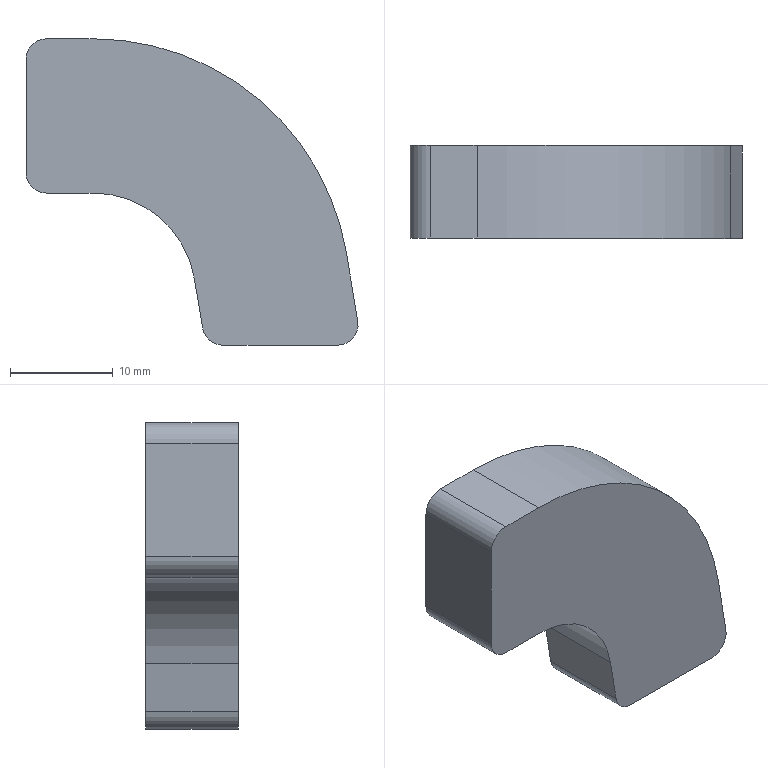Part | SolidWorks | features Fillet 1, FlatPattern 1, SMBaseFlange 1, SheetMetal 1 | 1 solid | 14 faces | box 32.296 x 9 x 29.799 mm | volume 5219 mm3 | plane 8 | cylinder 6 | commonest cylinder face diameters 4 x4 20 x1 50 x1
STEP:
#1=CARTESIAN_POINT('',(0.,0.,2.));
#2=VERTEX_POINT('',#1);
#3=CARTESIAN_POINT('',(0.,0.,13.));
#4=VERTEX_POINT('',#3);
#5=CARTESIAN_POINT('',(0.,0.,0.));
#6=DIRECTION('',(0.,0.,1.));
#7=VECTOR('',#6,1000.);
#8=LINE('',#5,#7);
#9=EDGE_CURVE('',#2,#4,#8,.T.);
#10=ORIENTED_EDGE('',*,*,#9,.T.);
#11=CARTESIAN_POINT('',(0.,9.,13.));
#12=VERTEX_POINT('',#11);
#13=CARTESIAN_POINT('',(0.,9.,13.));
#14=DIRECTION('',(0.,1.,0.));
#15=VECTOR('',#14,1000.);
#16=LINE('',#13,#15);
#17=EDGE_CURVE('',#4,#12,#16,.T.);
#18=ORIENTED_EDGE('',*,*,#17,.T.);
#19=CARTESIAN_POINT('',(0.,9.,2.));
#20=VERTEX_POINT('',#19);
#21=CARTESIAN_POINT('',(0.,9.,0.));
#22=DIRECTION('',(0.,0.,1.));
#23=VECTOR('',#22,1000.);
#24=LINE('',#21,#23);
#25=EDGE_CURVE('',#20,#12,#24,.T.);
#26=ORIENTED_EDGE('',*,*,#25,.F.);
#27=CARTESIAN_POINT('',(0.,9.,2.));
#28=DIRECTION('',(0.,-1.,0.));
#29=VECTOR('',#28,1000.);
#30=LINE('',#27,#29);
#31=EDGE_CURVE('',#20,#2,#30,.T.);
#32=ORIENTED_EDGE('',*,*,#31,.T.);
#33=EDGE_LOOP('',(#10,#18,#26,#32));
#34=FACE_OUTER_BOUND('',#33,.T.);
#35=CARTESIAN_POINT('',(0.,9.,0.));
#36=DIRECTION('',(1.,0.,0.));
#37=DIRECTION('',(0.,0.,-1.));
#38=AXIS2_PLACEMENT_3D('',#35,#36,#37);
#39=PLANE('',#38);
#40=ADVANCED_FACE('',(#34),#39,.F.);
#41=CARTESIAN_POINT('',(2.,9.,15.));
#42=VERTEX_POINT('',#41);
#43=CARTESIAN_POINT('',(6.519,9.,15.));
#44=VERTEX_POINT('',#43);
#45=CARTESIAN_POINT('',(0.,9.,15.));
#46=DIRECTION('',(1.,0.,0.));
#47=VECTOR('',#46,1000.);
#48=LINE('',#45,#47);
#49=EDGE_CURVE('',#42,#44,#48,.T.);
#50=ORIENTED_EDGE('',*,*,#49,.F.);
#51=CARTESIAN_POINT('',(2.,0.,15.));
#52=VERTEX_POINT('',#51);
#53=CARTESIAN_POINT('',(2.,9.,15.));
#54=DIRECTION('',(0.,-1.,0.));
#55=VECTOR('',#54,1000.);
#56=LINE('',#53,#55);
#57=EDGE_CURVE('',#42,#52,#56,.T.);
#58=ORIENTED_EDGE('',*,*,#57,.T.);
#59=CARTESIAN_POINT('',(6.519,0.,15.));
#60=VERTEX_POINT('',#59);
#61=CARTESIAN_POINT('',(0.,0.,15.));
#62=DIRECTION('',(1.,0.,0.));
#63=VECTOR('',#62,1000.);
#64=LINE('',#61,#63);
#65=EDGE_CURVE('',#52,#60,#64,.T.);
#66=ORIENTED_EDGE('',*,*,#65,.T.);
#67=CARTESIAN_POINT('',(6.519,9.,15.));
#68=DIRECTION('',(0.,-1.,0.));
#69=VECTOR('',#68,1000.);
#70=LINE('',#67,#69);
#71=EDGE_CURVE('',#44,#60,#70,.T.);
#72=ORIENTED_EDGE('',*,*,#71,.F.);
#73=EDGE_LOOP('',(#50,#58,#66,#72));
#74=FACE_OUTER_BOUND('',#73,.T.);
#75=CARTESIAN_POINT('',(0.,9.,15.));
#76=DIRECTION('',(0.,0.,-1.));
#77=DIRECTION('',(-1.,0.,0.));
#78=AXIS2_PLACEMENT_3D('',#75,#76,#77);
#79=PLANE('',#78);
#80=ADVANCED_FACE('',(#74),#79,.F.);
#81=CARTESIAN_POINT('',(31.184,0.,-5.917));
#82=VERTEX_POINT('',#81);
#83=CARTESIAN_POINT('',(6.519,0.,-10.));
#84=DIRECTION('',(0.,1.,0.));
#85=DIRECTION('',(0.,0.,1.));
#86=AXIS2_PLACEMENT_3D('',#83,#84,#85);
#87=CIRCLE('',#86,25.);
#88=EDGE_CURVE('',#60,#82,#87,.T.);
#89=ORIENTED_EDGE('',*,*,#88,.T.);
#90=CARTESIAN_POINT('',(31.184,9.,-5.917));
#91=VERTEX_POINT('',#90);
#92=CARTESIAN_POINT('',(31.184,9.,-5.917));
#93=DIRECTION('',(0.,-1.,0.));
#94=VECTOR('',#93,1000.);
#95=LINE('',#92,#94);
#96=EDGE_CURVE('',#91,#82,#95,.T.);
#97=ORIENTED_EDGE('',*,*,#96,.F.);
#98=CARTESIAN_POINT('',(6.519,9.,-10.));
#99=DIRECTION('',(0.,1.,0.));
#100=DIRECTION('',(0.,0.,1.));
#101=AXIS2_PLACEMENT_3D('',#98,#99,#100);
#102=CIRCLE('',#101,25.);
#103=EDGE_CURVE('',#44,#91,#102,.T.);
#104=ORIENTED_EDGE('',*,*,#103,.F.);
#105=ORIENTED_EDGE('',*,*,#71,.T.);
#106=EDGE_LOOP('',(#89,#97,#104,#105));
#107=FACE_OUTER_BOUND('',#106,.T.);
#108=CARTESIAN_POINT('',(6.519,9.,-10.));
#109=DIRECTION('',(0.,-1.,0.));
#110=DIRECTION('',(0.,0.,-1.));
#111=AXIS2_PLACEMENT_3D('',#108,#109,#110);
#112=CYLINDRICAL_SURFACE('',#111,25.);
#113=ADVANCED_FACE('',(#107),#112,.T.);
#114=CARTESIAN_POINT('',(32.269,0.,-12.472));
#115=VERTEX_POINT('',#114);
#116=CARTESIAN_POINT('',(31.184,0.,-5.917));
#117=DIRECTION('',(0.1633,0.,-0.9866));
#118=VECTOR('',#117,1000.);
#119=LINE('',#116,#118);
#120=EDGE_CURVE('',#82,#115,#119,.T.);
#121=ORIENTED_EDGE('',*,*,#120,.T.);
#122=CARTESIAN_POINT('',(32.269,9.,-12.472));
#123=VERTEX_POINT('',#122);
#124=CARTESIAN_POINT('',(32.269,9.,-12.472));
#125=DIRECTION('',(0.,1.,0.));
#126=VECTOR('',#125,1000.);
#127=LINE('',#124,#126);
#128=EDGE_CURVE('',#115,#123,#127,.T.);
#129=ORIENTED_EDGE('',*,*,#128,.T.);
#130=CARTESIAN_POINT('',(31.184,9.,-5.917));
#131=DIRECTION('',(0.1633,0.,-0.9866));
#132=VECTOR('',#131,1000.);
#133=LINE('',#130,#132);
#134=EDGE_CURVE('',#91,#123,#133,.T.);
#135=ORIENTED_EDGE('',*,*,#134,.F.);
#136=ORIENTED_EDGE('',*,*,#96,.T.);
#137=EDGE_LOOP('',(#121,#129,#135,#136));
#138=FACE_OUTER_BOUND('',#137,.T.);
#139=CARTESIAN_POINT('',(31.184,9.,-5.917));
#140=DIRECTION('',(-0.9866,0.,-0.1633));
#141=DIRECTION('',(-0.1633,0.,0.9866));
#142=AXIS2_PLACEMENT_3D('',#139,#140,#141);
#143=PLANE('',#142);
#144=ADVANCED_FACE('',(#138),#143,.F.);
#145=CARTESIAN_POINT('',(30.296,9.,-14.799));
#146=VERTEX_POINT('',#145);
#147=CARTESIAN_POINT('',(19.146,9.,-14.799));
#148=VERTEX_POINT('',#147);
#149=CARTESIAN_POINT('',(17.45,9.,-14.799));
#150=DIRECTION('',(-1.,0.,0.));
#151=VECTOR('',#150,1000.);
#152=LINE('',#149,#151);
#153=EDGE_CURVE('',#146,#148,#152,.T.);
#154=ORIENTED_EDGE('',*,*,#153,.F.);
#155=CARTESIAN_POINT('',(30.296,0.,-14.799));
#156=VERTEX_POINT('',#155);
#157=CARTESIAN_POINT('',(30.296,9.,-14.799));
#158=DIRECTION('',(0.,-1.,0.));
#159=VECTOR('',#158,1000.);
#160=LINE('',#157,#159);
#161=EDGE_CURVE('',#146,#156,#160,.T.);
#162=ORIENTED_EDGE('',*,*,#161,.T.);
#163=CARTESIAN_POINT('',(19.146,0.,-14.799));
#164=VERTEX_POINT('',#163);
#165=CARTESIAN_POINT('',(17.45,0.,-14.799));
#166=DIRECTION('',(-1.,0.,0.));
#167=VECTOR('',#166,1000.);
#168=LINE('',#165,#167);
#169=EDGE_CURVE('',#156,#164,#168,.T.);
#170=ORIENTED_EDGE('',*,*,#169,.T.);
#171=CARTESIAN_POINT('',(19.146,9.,-14.799));
#172=DIRECTION('',(0.,1.,0.));
#173=VECTOR('',#172,1000.);
#174=LINE('',#171,#173);
#175=EDGE_CURVE('',#164,#148,#174,.T.);
#176=ORIENTED_EDGE('',*,*,#175,.T.);
#177=EDGE_LOOP('',(#154,#162,#170,#176));
#178=FACE_OUTER_BOUND('',#177,.T.);
#179=CARTESIAN_POINT('',(17.45,9.,-14.799));
#180=DIRECTION('',(0.,0.,1.));
#181=DIRECTION('',(1.,0.,0.));
#182=AXIS2_PLACEMENT_3D('',#179,#180,#181);
#183=PLANE('',#182);
#184=ADVANCED_FACE('',(#178),#183,.F.);
#185=CARTESIAN_POINT('',(17.173,9.,-13.125));
#186=VERTEX_POINT('',#185);
#187=CARTESIAN_POINT('',(16.385,9.,-8.367));
#188=VERTEX_POINT('',#187);
#189=CARTESIAN_POINT('',(16.385,9.,-8.367));
#190=DIRECTION('',(-0.1633,0.,0.9866));
#191=VECTOR('',#190,1000.);
#192=LINE('',#189,#191);
#193=EDGE_CURVE('',#186,#188,#192,.T.);
#194=ORIENTED_EDGE('',*,*,#193,.F.);
#195=CARTESIAN_POINT('',(17.173,0.,-13.125));
#196=VERTEX_POINT('',#195);
#197=CARTESIAN_POINT('',(17.173,9.,-13.125));
#198=DIRECTION('',(0.,-1.,0.));
#199=VECTOR('',#198,1000.);
#200=LINE('',#197,#199);
#201=EDGE_CURVE('',#186,#196,#200,.T.);
#202=ORIENTED_EDGE('',*,*,#201,.T.);
#203=CARTESIAN_POINT('',(16.385,0.,-8.367));
#204=VERTEX_POINT('',#203);
#205=CARTESIAN_POINT('',(16.385,0.,-8.367));
#206=DIRECTION('',(-0.1633,0.,0.9866));
#207=VECTOR('',#206,1000.);
#208=LINE('',#205,#207);
#209=EDGE_CURVE('',#196,#204,#208,.T.);
#210=ORIENTED_EDGE('',*,*,#209,.T.);
#211=CARTESIAN_POINT('',(16.385,9.,-8.367));
#212=DIRECTION('',(0.,-1.,0.));
#213=VECTOR('',#212,1000.);
#214=LINE('',#211,#213);
#215=EDGE_CURVE('',#188,#204,#214,.T.);
#216=ORIENTED_EDGE('',*,*,#215,.F.);
#217=EDGE_LOOP('',(#194,#202,#210,#216));
#218=FACE_OUTER_BOUND('',#217,.T.);
#219=CARTESIAN_POINT('',(16.385,9.,-8.367));
#220=DIRECTION('',(0.9866,0.,0.1633));
#221=DIRECTION('',(0.1633,0.,-0.9866));
#222=AXIS2_PLACEMENT_3D('',#219,#220,#221);
#223=PLANE('',#222);
#224=ADVANCED_FACE('',(#218),#223,.F.);
#225=CARTESIAN_POINT('',(6.519,0.,0.));
#226=VERTEX_POINT('',#225);
#227=CARTESIAN_POINT('',(6.519,0.,-10.));
#228=DIRECTION('',(0.,-1.,0.));
#229=DIRECTION('',(0.,0.,1.));
#230=AXIS2_PLACEMENT_3D('',#227,#228,#229);
#231=CIRCLE('',#230,10.);
#232=EDGE_CURVE('',#204,#226,#231,.T.);
#233=ORIENTED_EDGE('',*,*,#232,.T.);
#234=CARTESIAN_POINT('',(6.519,9.,0.));
#235=VERTEX_POINT('',#234);
#236=CARTESIAN_POINT('',(6.519,9.,0.));
#237=DIRECTION('',(0.,-1.,0.));
#238=VECTOR('',#237,1000.);
#239=LINE('',#236,#238);
#240=EDGE_CURVE('',#235,#226,#239,.T.);
#241=ORIENTED_EDGE('',*,*,#240,.F.);
#242=CARTESIAN_POINT('',(6.519,9.,-10.));
#243=DIRECTION('',(0.,-1.,0.));
#244=DIRECTION('',(0.,0.,1.));
#245=AXIS2_PLACEMENT_3D('',#242,#243,#244);
#246=CIRCLE('',#245,10.);
#247=EDGE_CURVE('',#188,#235,#246,.T.);
#248=ORIENTED_EDGE('',*,*,#247,.F.);
#249=ORIENTED_EDGE('',*,*,#215,.T.);
#250=EDGE_LOOP('',(#233,#241,#248,#249));
#251=FACE_OUTER_BOUND('',#250,.T.);
#252=CARTESIAN_POINT('',(6.519,9.,-10.));
#253=DIRECTION('',(0.,-1.,0.));
#254=DIRECTION('',(0.,0.,-1.));
#255=AXIS2_PLACEMENT_3D('',#252,#253,#254);
#256=CYLINDRICAL_SURFACE('',#255,10.);
#257=ADVANCED_FACE('',(#251),#256,.F.);
#258=CARTESIAN_POINT('',(2.,0.,0.));
#259=VERTEX_POINT('',#258);
#260=CARTESIAN_POINT('',(0.,0.,0.));
#261=DIRECTION('',(-1.,0.,0.));
#262=VECTOR('',#261,1000.);
#263=LINE('',#260,#262);
#264=EDGE_CURVE('',#226,#259,#263,.T.);
#265=ORIENTED_EDGE('',*,*,#264,.T.);
#266=CARTESIAN_POINT('',(2.,9.,0.));
#267=VERTEX_POINT('',#266);
#268=CARTESIAN_POINT('',(2.,9.,0.));
#269=DIRECTION('',(0.,1.,0.));
#270=VECTOR('',#269,1000.);
#271=LINE('',#268,#270);
#272=EDGE_CURVE('',#259,#267,#271,.T.);
#273=ORIENTED_EDGE('',*,*,#272,.T.);
#274=CARTESIAN_POINT('',(0.,9.,0.));
#275=DIRECTION('',(-1.,0.,0.));
#276=VECTOR('',#275,1000.);
#277=LINE('',#274,#276);
#278=EDGE_CURVE('',#235,#267,#277,.T.);
#279=ORIENTED_EDGE('',*,*,#278,.F.);
#280=ORIENTED_EDGE('',*,*,#240,.T.);
#281=EDGE_LOOP('',(#265,#273,#279,#280));
#282=FACE_OUTER_BOUND('',#281,.T.);
#283=CARTESIAN_POINT('',(0.,9.,0.));
#284=DIRECTION('',(0.,0.,1.));
#285=DIRECTION('',(1.,0.,0.));
#286=AXIS2_PLACEMENT_3D('',#283,#284,#285);
#287=PLANE('',#286);
#288=ADVANCED_FACE('',(#282),#287,.F.);
#289=ORIENTED_EDGE('',*,*,#134,.T.);
#290=CARTESIAN_POINT('',(30.296,9.,-12.799));
#291=DIRECTION('',(0.,1.,0.));
#292=DIRECTION('',(0.,0.,1.));
#293=AXIS2_PLACEMENT_3D('',#290,#291,#292);
#294=CIRCLE('',#293,2.);
#295=EDGE_CURVE('',#123,#146,#294,.T.);
#296=ORIENTED_EDGE('',*,*,#295,.T.);
#297=ORIENTED_EDGE('',*,*,#153,.T.);
#298=CARTESIAN_POINT('',(19.146,9.,-12.799));
#299=DIRECTION('',(0.,1.,0.));
#300=DIRECTION('',(0.,0.,1.));
#301=AXIS2_PLACEMENT_3D('',#298,#299,#300);
#302=CIRCLE('',#301,2.);
#303=EDGE_CURVE('',#148,#186,#302,.T.);
#304=ORIENTED_EDGE('',*,*,#303,.T.);
#305=ORIENTED_EDGE('',*,*,#193,.T.);
#306=ORIENTED_EDGE('',*,*,#247,.T.);
#307=ORIENTED_EDGE('',*,*,#278,.T.);
#308=CARTESIAN_POINT('',(2.,9.,2.));
#309=DIRECTION('',(0.,1.,0.));
#310=DIRECTION('',(0.,0.,1.));
#311=AXIS2_PLACEMENT_3D('',#308,#309,#310);
#312=CIRCLE('',#311,2.);
#313=EDGE_CURVE('',#267,#20,#312,.T.);
#314=ORIENTED_EDGE('',*,*,#313,.T.);
#315=ORIENTED_EDGE('',*,*,#25,.T.);
#316=CARTESIAN_POINT('',(2.,9.,13.));
#317=DIRECTION('',(0.,1.,0.));
#318=DIRECTION('',(0.,0.,1.));
#319=AXIS2_PLACEMENT_3D('',#316,#317,#318);
#320=CIRCLE('',#319,2.);
#321=EDGE_CURVE('',#12,#42,#320,.T.);
#322=ORIENTED_EDGE('',*,*,#321,.T.);
#323=ORIENTED_EDGE('',*,*,#49,.T.);
#324=ORIENTED_EDGE('',*,*,#103,.T.);
#325=EDGE_LOOP('',(#289,#296,#297,#304,#305,#306,#307,#314,#315,#322,#323,#324));
#326=FACE_OUTER_BOUND('',#325,.T.);
#327=CARTESIAN_POINT('',(6.519,9.,-10.));
#328=DIRECTION('',(0.,1.,0.));
#329=DIRECTION('',(0.,0.,1.));
#330=AXIS2_PLACEMENT_3D('',#327,#328,#329);
#331=PLANE('',#330);
#332=ADVANCED_FACE('',(#326),#331,.T.);
#333=ORIENTED_EDGE('',*,*,#169,.F.);
#334=CARTESIAN_POINT('',(30.296,0.,-12.799));
#335=DIRECTION('',(0.,-1.,0.));
#336=DIRECTION('',(0.,0.,1.));
#337=AXIS2_PLACEMENT_3D('',#334,#335,#336);
#338=CIRCLE('',#337,2.);
#339=EDGE_CURVE('',#156,#115,#338,.T.);
#340=ORIENTED_EDGE('',*,*,#339,.T.);
#341=ORIENTED_EDGE('',*,*,#120,.F.);
#342=ORIENTED_EDGE('',*,*,#88,.F.);
#343=ORIENTED_EDGE('',*,*,#65,.F.);
#344=CARTESIAN_POINT('',(2.,0.,13.));
#345=DIRECTION('',(0.,-1.,0.));
#346=DIRECTION('',(0.,0.,1.));
#347=AXIS2_PLACEMENT_3D('',#344,#345,#346);
#348=CIRCLE('',#347,2.);
#349=EDGE_CURVE('',#52,#4,#348,.T.);
#350=ORIENTED_EDGE('',*,*,#349,.T.);
#351=ORIENTED_EDGE('',*,*,#9,.F.);
#352=CARTESIAN_POINT('',(2.,0.,2.));
#353=DIRECTION('',(0.,-1.,0.));
#354=DIRECTION('',(0.,0.,1.));
#355=AXIS2_PLACEMENT_3D('',#352,#353,#354);
#356=CIRCLE('',#355,2.);
#357=EDGE_CURVE('',#2,#259,#356,.T.);
#358=ORIENTED_EDGE('',*,*,#357,.T.);
#359=ORIENTED_EDGE('',*,*,#264,.F.);
#360=ORIENTED_EDGE('',*,*,#232,.F.);
#361=ORIENTED_EDGE('',*,*,#209,.F.);
#362=CARTESIAN_POINT('',(19.146,0.,-12.799));
#363=DIRECTION('',(0.,-1.,0.));
#364=DIRECTION('',(0.,0.,1.));
#365=AXIS2_PLACEMENT_3D('',#362,#363,#364);
#366=CIRCLE('',#365,2.);
#367=EDGE_CURVE('',#196,#164,#366,.T.);
#368=ORIENTED_EDGE('',*,*,#367,.T.);
#369=EDGE_LOOP('',(#333,#340,#341,#342,#343,#350,#351,#358,#359,#360,#361,#368));
#370=FACE_OUTER_BOUND('',#369,.T.);
#371=CARTESIAN_POINT('',(6.519,0.,-10.));
#372=DIRECTION('',(0.,1.,0.));
#373=DIRECTION('',(0.,0.,1.));
#374=AXIS2_PLACEMENT_3D('',#371,#372,#373);
#375=PLANE('',#374);
#376=ADVANCED_FACE('',(#370),#375,.F.);
#377=ORIENTED_EDGE('',*,*,#295,.F.);
#378=ORIENTED_EDGE('',*,*,#128,.F.);
#379=ORIENTED_EDGE('',*,*,#339,.F.);
#380=ORIENTED_EDGE('',*,*,#161,.F.);
#381=EDGE_LOOP('',(#377,#378,#379,#380));
#382=FACE_OUTER_BOUND('',#381,.T.);
#383=CARTESIAN_POINT('',(30.296,9.,-12.799));
#384=DIRECTION('',(0.,-1.,0.));
#385=DIRECTION('',(0.,0.,-1.));
#386=AXIS2_PLACEMENT_3D('',#383,#384,#385);
#387=CYLINDRICAL_SURFACE('',#386,2.);
#388=ADVANCED_FACE('',(#382),#387,.T.);
#389=ORIENTED_EDGE('',*,*,#303,.F.);
#390=ORIENTED_EDGE('',*,*,#175,.F.);
#391=ORIENTED_EDGE('',*,*,#367,.F.);
#392=ORIENTED_EDGE('',*,*,#201,.F.);
#393=EDGE_LOOP('',(#389,#390,#391,#392));
#394=FACE_OUTER_BOUND('',#393,.T.);
#395=CARTESIAN_POINT('',(19.146,9.,-12.799));
#396=DIRECTION('',(0.,-1.,0.));
#397=DIRECTION('',(0.,0.,-1.));
#398=AXIS2_PLACEMENT_3D('',#395,#396,#397);
#399=CYLINDRICAL_SURFACE('',#398,2.);
#400=ADVANCED_FACE('',(#394),#399,.T.);
#401=ORIENTED_EDGE('',*,*,#321,.F.);
#402=ORIENTED_EDGE('',*,*,#17,.F.);
#403=ORIENTED_EDGE('',*,*,#349,.F.);
#404=ORIENTED_EDGE('',*,*,#57,.F.);
#405=EDGE_LOOP('',(#401,#402,#403,#404));
#406=FACE_OUTER_BOUND('',#405,.T.);
#407=CARTESIAN_POINT('',(2.,9.,13.));
#408=DIRECTION('',(0.,-1.,0.));
#409=DIRECTION('',(0.,0.,-1.));
#410=AXIS2_PLACEMENT_3D('',#407,#408,#409);
#411=CYLINDRICAL_SURFACE('',#410,2.);
#412=ADVANCED_FACE('',(#406),#411,.T.);
#413=ORIENTED_EDGE('',*,*,#313,.F.);
#414=ORIENTED_EDGE('',*,*,#272,.F.);
#415=ORIENTED_EDGE('',*,*,#357,.F.);
#416=ORIENTED_EDGE('',*,*,#31,.F.);
#417=EDGE_LOOP('',(#413,#414,#415,#416));
#418=FACE_OUTER_BOUND('',#417,.T.);
#419=CARTESIAN_POINT('',(2.,9.,2.));
#420=DIRECTION('',(0.,-1.,0.));
#421=DIRECTION('',(0.,0.,-1.));
#422=AXIS2_PLACEMENT_3D('',#419,#420,#421);
#423=CYLINDRICAL_SURFACE('',#422,2.);
#424=ADVANCED_FACE('',(#418),#423,.T.);
#425=CLOSED_SHELL('',(#40,#80,#113,#144,#184,#224,#257,#288,#332,#376,#388,#400,#412,#424));
#426=MANIFOLD_SOLID_BREP('',#425);
#427=CARTESIAN_POINT('',(0.,0.,0.));
#428=DIRECTION('',(0.,0.,1.));
#429=DIRECTION('',(1.,0.,0.));
#430=AXIS2_PLACEMENT_3D('',#427,#428,#429);
#431=(LENGTH_UNIT()NAMED_UNIT(*)SI_UNIT(.MILLI.,.METRE.));
#432=UNCERTAINTY_MEASURE_WITH_UNIT(LENGTH_MEASURE(0.00001),#431,'','');
#433=(NAMED_UNIT(*)PLANE_ANGLE_UNIT()SI_UNIT($,.RADIAN.));
#434=(NAMED_UNIT(*)SI_UNIT($,.STERADIAN.)SOLID_ANGLE_UNIT());
#435=(GEOMETRIC_REPRESENTATION_CONTEXT(3)GLOBAL_UNCERTAINTY_ASSIGNED_CONTEXT((#432))GLOBAL_UNIT_ASSIGNED_CONTEXT((#431,#433,#434))REPRESENTATION_CONTEXT('',''));
#436=ADVANCED_BREP_SHAPE_REPRESENTATION('',(#426,#430),#435);